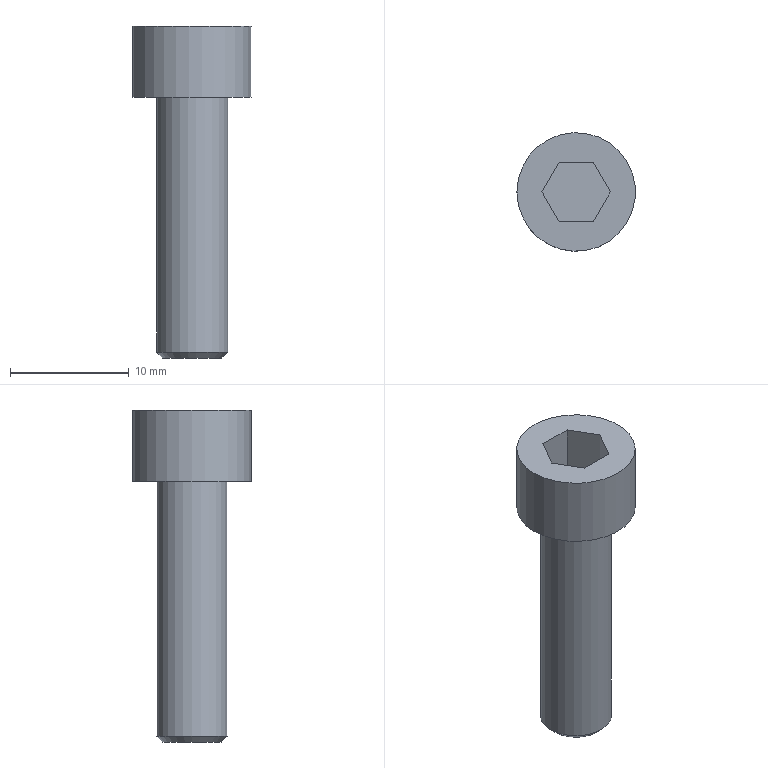Part | STEP file | solid 33 | 1 solid | 13 faces | box 10 x 10 x 28 mm | volume 1005 mm3 | plane 10 | cylinder 2 | cone 1 | commonest cylinder face diameters 6 x1 10 x1